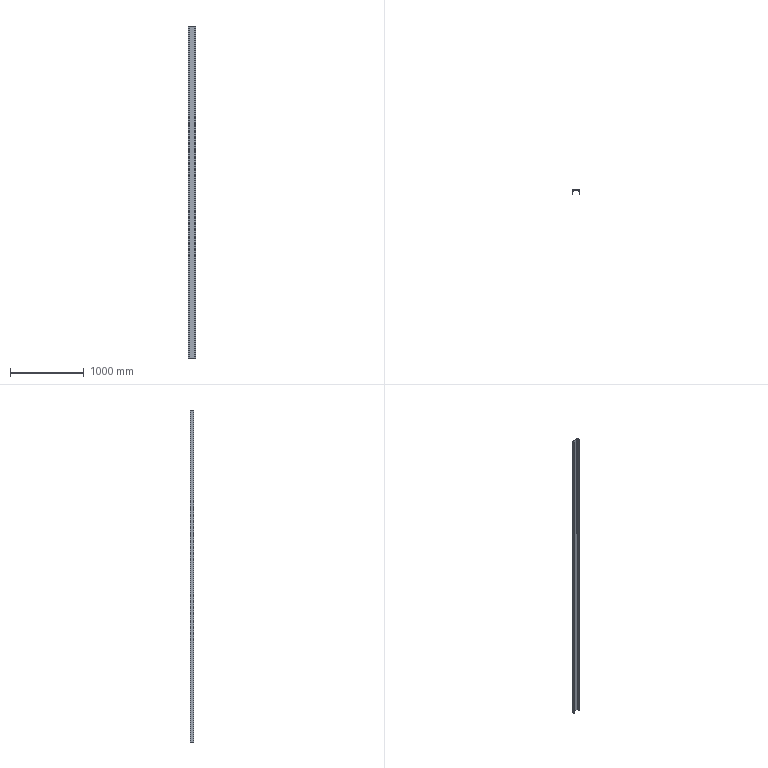Part | SolidWorks | features Extrusion 1 | 1 solid | 14 faces | box 100 x 50 x 4500 mm | volume 5749980 mm3 | plane 10 | cylinder 4 | commonest cylinder face diameters 4 x2 10 x2
STEP:
#1=CARTESIAN_POINT('',(0.,0.,0.));
#2=VERTEX_POINT('',#1);
#3=CARTESIAN_POINT('',(2.549,0.,0.));
#4=VERTEX_POINT('',#3);
#5=CARTESIAN_POINT('',(0.,0.,0.));
#6=DIRECTION('',(1.,0.,0.));
#7=VECTOR('',#6,1000.);
#8=LINE('',#5,#7);
#9=EDGE_CURVE('',#2,#4,#8,.T.);
#10=ORIENTED_EDGE('',*,*,#9,.T.);
#11=CARTESIAN_POINT('',(2.549,0.,4500.));
#12=VERTEX_POINT('',#11);
#13=CARTESIAN_POINT('',(2.549,0.,4500.));
#14=DIRECTION('',(0.,0.,-1.));
#15=VECTOR('',#14,1000.);
#16=LINE('',#13,#15);
#17=EDGE_CURVE('',#12,#4,#16,.T.);
#18=ORIENTED_EDGE('',*,*,#17,.F.);
#19=CARTESIAN_POINT('',(0.,0.,4500.));
#20=VERTEX_POINT('',#19);
#21=CARTESIAN_POINT('',(0.,0.,4500.));
#22=DIRECTION('',(1.,0.,0.));
#23=VECTOR('',#22,1000.);
#24=LINE('',#21,#23);
#25=EDGE_CURVE('',#20,#12,#24,.T.);
#26=ORIENTED_EDGE('',*,*,#25,.F.);
#27=CARTESIAN_POINT('',(0.,0.,4500.));
#28=DIRECTION('',(0.,0.,-1.));
#29=VECTOR('',#28,1000.);
#30=LINE('',#27,#29);
#31=EDGE_CURVE('',#20,#2,#30,.T.);
#32=ORIENTED_EDGE('',*,*,#31,.T.);
#33=EDGE_LOOP('',(#10,#18,#26,#32));
#34=FACE_OUTER_BOUND('',#33,.T.);
#35=CARTESIAN_POINT('',(0.,0.,4500.));
#36=DIRECTION('',(0.,1.,0.));
#37=DIRECTION('',(0.,0.,1.));
#38=AXIS2_PLACEMENT_3D('',#35,#36,#37);
#39=PLANE('',#38);
#40=ADVANCED_FACE('',(#34),#39,.F.);
#41=CARTESIAN_POINT('',(4.536,1.773,0.));
#42=VERTEX_POINT('',#41);
#43=CARTESIAN_POINT('',(2.549,2.,0.));
#44=DIRECTION('',(0.,0.,1.));
#45=DIRECTION('',(-1.,0.,0.));
#46=AXIS2_PLACEMENT_3D('',#43,#44,#45);
#47=CIRCLE('',#46,2.);
#48=EDGE_CURVE('',#4,#42,#47,.T.);
#49=ORIENTED_EDGE('',*,*,#48,.T.);
#50=CARTESIAN_POINT('',(4.536,1.773,4500.));
#51=VERTEX_POINT('',#50);
#52=CARTESIAN_POINT('',(4.536,1.773,4500.));
#53=DIRECTION('',(0.,0.,-1.));
#54=VECTOR('',#53,1000.);
#55=LINE('',#52,#54);
#56=EDGE_CURVE('',#51,#42,#55,.T.);
#57=ORIENTED_EDGE('',*,*,#56,.F.);
#58=CARTESIAN_POINT('',(2.549,2.,4500.));
#59=DIRECTION('',(0.,0.,1.));
#60=DIRECTION('',(-1.,0.,0.));
#61=AXIS2_PLACEMENT_3D('',#58,#59,#60);
#62=CIRCLE('',#61,2.);
#63=EDGE_CURVE('',#12,#51,#62,.T.);
#64=ORIENTED_EDGE('',*,*,#63,.F.);
#65=ORIENTED_EDGE('',*,*,#17,.T.);
#66=EDGE_LOOP('',(#49,#57,#64,#65));
#67=FACE_OUTER_BOUND('',#66,.T.);
#68=CARTESIAN_POINT('',(2.549,2.,4500.));
#69=DIRECTION('',(0.,0.,-1.));
#70=DIRECTION('',(-1.,0.,0.));
#71=AXIS2_PLACEMENT_3D('',#68,#69,#70);
#72=CYLINDRICAL_SURFACE('',#71,2.);
#73=ADVANCED_FACE('',(#67),#72,.T.);
#74=CARTESIAN_POINT('',(8.753,38.724,0.));
#75=VERTEX_POINT('',#74);
#76=CARTESIAN_POINT('',(4.536,1.773,0.));
#77=DIRECTION('',(0.1134,0.9936,0.));
#78=VECTOR('',#77,1000.);
#79=LINE('',#76,#78);
#80=EDGE_CURVE('',#42,#75,#79,.T.);
#81=ORIENTED_EDGE('',*,*,#80,.T.);
#82=CARTESIAN_POINT('',(8.753,38.724,4500.));
#83=VERTEX_POINT('',#82);
#84=CARTESIAN_POINT('',(8.753,38.724,4500.));
#85=DIRECTION('',(0.,0.,-1.));
#86=VECTOR('',#85,1000.);
#87=LINE('',#84,#86);
#88=EDGE_CURVE('',#83,#75,#87,.T.);
#89=ORIENTED_EDGE('',*,*,#88,.F.);
#90=CARTESIAN_POINT('',(4.536,1.773,4500.));
#91=DIRECTION('',(0.1134,0.9936,0.));
#92=VECTOR('',#91,1000.);
#93=LINE('',#90,#92);
#94=EDGE_CURVE('',#51,#83,#93,.T.);
#95=ORIENTED_EDGE('',*,*,#94,.F.);
#96=ORIENTED_EDGE('',*,*,#56,.T.);
#97=EDGE_LOOP('',(#81,#89,#95,#96));
#98=FACE_OUTER_BOUND('',#97,.T.);
#99=CARTESIAN_POINT('',(4.536,1.773,4500.));
#100=DIRECTION('',(-0.9936,0.1134,0.));
#101=DIRECTION('',(-0.1134,-0.9936,0.));
#102=AXIS2_PLACEMENT_3D('',#99,#100,#101);
#103=PLANE('',#102);
#104=ADVANCED_FACE('',(#98),#103,.F.);
#105=CARTESIAN_POINT('',(13.72,43.157,0.));
#106=VERTEX_POINT('',#105);
#107=CARTESIAN_POINT('',(13.72,38.157,0.));
#108=DIRECTION('',(0.,0.,-1.));
#109=DIRECTION('',(-1.,0.,0.));
#110=AXIS2_PLACEMENT_3D('',#107,#108,#109);
#111=CIRCLE('',#110,5.);
#112=EDGE_CURVE('',#75,#106,#111,.T.);
#113=ORIENTED_EDGE('',*,*,#112,.T.);
#114=CARTESIAN_POINT('',(13.72,43.157,4500.));
#115=VERTEX_POINT('',#114);
#116=CARTESIAN_POINT('',(13.72,43.157,4500.));
#117=DIRECTION('',(0.,0.,-1.));
#118=VECTOR('',#117,1000.);
#119=LINE('',#116,#118);
#120=EDGE_CURVE('',#115,#106,#119,.T.);
#121=ORIENTED_EDGE('',*,*,#120,.F.);
#122=CARTESIAN_POINT('',(13.72,38.157,4500.));
#123=DIRECTION('',(0.,0.,-1.));
#124=DIRECTION('',(-1.,0.,0.));
#125=AXIS2_PLACEMENT_3D('',#122,#123,#124);
#126=CIRCLE('',#125,5.);
#127=EDGE_CURVE('',#83,#115,#126,.T.);
#128=ORIENTED_EDGE('',*,*,#127,.F.);
#129=ORIENTED_EDGE('',*,*,#88,.T.);
#130=EDGE_LOOP('',(#113,#121,#128,#129));
#131=FACE_OUTER_BOUND('',#130,.T.);
#132=CARTESIAN_POINT('',(13.72,38.157,4500.));
#133=DIRECTION('',(0.,0.,-1.));
#134=DIRECTION('',(-1.,0.,0.));
#135=AXIS2_PLACEMENT_3D('',#132,#133,#134);
#136=CYLINDRICAL_SURFACE('',#135,5.);
#137=ADVANCED_FACE('',(#131),#136,.F.);
#138=CARTESIAN_POINT('',(86.28,43.157,0.));
#139=VERTEX_POINT('',#138);
#140=CARTESIAN_POINT('',(13.72,43.157,0.));
#141=DIRECTION('',(1.,0.,0.));
#142=VECTOR('',#141,1000.);
#143=LINE('',#140,#142);
#144=EDGE_CURVE('',#106,#139,#143,.T.);
#145=ORIENTED_EDGE('',*,*,#144,.T.);
#146=CARTESIAN_POINT('',(86.28,43.157,4500.));
#147=VERTEX_POINT('',#146);
#148=CARTESIAN_POINT('',(86.28,43.157,4500.));
#149=DIRECTION('',(0.,0.,-1.));
#150=VECTOR('',#149,1000.);
#151=LINE('',#148,#150);
#152=EDGE_CURVE('',#147,#139,#151,.T.);
#153=ORIENTED_EDGE('',*,*,#152,.F.);
#154=CARTESIAN_POINT('',(13.72,43.157,4500.));
#155=DIRECTION('',(1.,0.,0.));
#156=VECTOR('',#155,1000.);
#157=LINE('',#154,#156);
#158=EDGE_CURVE('',#115,#147,#157,.T.);
#159=ORIENTED_EDGE('',*,*,#158,.F.);
#160=ORIENTED_EDGE('',*,*,#120,.T.);
#161=EDGE_LOOP('',(#145,#153,#159,#160));
#162=FACE_OUTER_BOUND('',#161,.T.);
#163=CARTESIAN_POINT('',(13.72,43.157,4500.));
#164=DIRECTION('',(0.,1.,0.));
#165=DIRECTION('',(-1.,0.,0.));
#166=AXIS2_PLACEMENT_3D('',#163,#164,#165);
#167=PLANE('',#166);
#168=ADVANCED_FACE('',(#162),#167,.F.);
#169=CARTESIAN_POINT('',(91.247,38.724,0.));
#170=VERTEX_POINT('',#169);
#171=CARTESIAN_POINT('',(86.28,38.157,0.));
#172=DIRECTION('',(0.,0.,-1.));
#173=DIRECTION('',(1.,0.,0.));
#174=AXIS2_PLACEMENT_3D('',#171,#172,#173);
#175=CIRCLE('',#174,5.);
#176=EDGE_CURVE('',#139,#170,#175,.T.);
#177=ORIENTED_EDGE('',*,*,#176,.T.);
#178=CARTESIAN_POINT('',(91.247,38.724,4500.));
#179=VERTEX_POINT('',#178);
#180=CARTESIAN_POINT('',(91.247,38.724,4500.));
#181=DIRECTION('',(0.,0.,-1.));
#182=VECTOR('',#181,1000.);
#183=LINE('',#180,#182);
#184=EDGE_CURVE('',#179,#170,#183,.T.);
#185=ORIENTED_EDGE('',*,*,#184,.F.);
#186=CARTESIAN_POINT('',(86.28,38.157,4500.));
#187=DIRECTION('',(0.,0.,-1.));
#188=DIRECTION('',(1.,0.,0.));
#189=AXIS2_PLACEMENT_3D('',#186,#187,#188);
#190=CIRCLE('',#189,5.);
#191=EDGE_CURVE('',#147,#179,#190,.T.);
#192=ORIENTED_EDGE('',*,*,#191,.F.);
#193=ORIENTED_EDGE('',*,*,#152,.T.);
#194=EDGE_LOOP('',(#177,#185,#192,#193));
#195=FACE_OUTER_BOUND('',#194,.T.);
#196=CARTESIAN_POINT('',(86.28,38.157,4500.));
#197=DIRECTION('',(0.,0.,-1.));
#198=DIRECTION('',(-1.,0.,0.));
#199=AXIS2_PLACEMENT_3D('',#196,#197,#198);
#200=CYLINDRICAL_SURFACE('',#199,5.);
#201=ADVANCED_FACE('',(#195),#200,.F.);
#202=CARTESIAN_POINT('',(95.464,1.773,0.));
#203=VERTEX_POINT('',#202);
#204=CARTESIAN_POINT('',(95.464,1.773,0.));
#205=DIRECTION('',(0.1134,-0.9936,0.));
#206=VECTOR('',#205,1000.);
#207=LINE('',#204,#206);
#208=EDGE_CURVE('',#170,#203,#207,.T.);
#209=ORIENTED_EDGE('',*,*,#208,.T.);
#210=CARTESIAN_POINT('',(95.464,1.773,4500.));
#211=VERTEX_POINT('',#210);
#212=CARTESIAN_POINT('',(95.464,1.773,4500.));
#213=DIRECTION('',(0.,0.,-1.));
#214=VECTOR('',#213,1000.);
#215=LINE('',#212,#214);
#216=EDGE_CURVE('',#211,#203,#215,.T.);
#217=ORIENTED_EDGE('',*,*,#216,.F.);
#218=CARTESIAN_POINT('',(95.464,1.773,4500.));
#219=DIRECTION('',(0.1134,-0.9936,0.));
#220=VECTOR('',#219,1000.);
#221=LINE('',#218,#220);
#222=EDGE_CURVE('',#179,#211,#221,.T.);
#223=ORIENTED_EDGE('',*,*,#222,.F.);
#224=ORIENTED_EDGE('',*,*,#184,.T.);
#225=EDGE_LOOP('',(#209,#217,#223,#224));
#226=FACE_OUTER_BOUND('',#225,.T.);
#227=CARTESIAN_POINT('',(95.464,1.773,4500.));
#228=DIRECTION('',(0.9936,0.1134,0.));
#229=DIRECTION('',(-0.1134,0.9936,0.));
#230=AXIS2_PLACEMENT_3D('',#227,#228,#229);
#231=PLANE('',#230);
#232=ADVANCED_FACE('',(#226),#231,.F.);
#233=CARTESIAN_POINT('',(97.451,0.,0.));
#234=VERTEX_POINT('',#233);
#235=CARTESIAN_POINT('',(97.451,2.,0.));
#236=DIRECTION('',(0.,0.,1.));
#237=DIRECTION('',(1.,0.,0.));
#238=AXIS2_PLACEMENT_3D('',#235,#236,#237);
#239=CIRCLE('',#238,2.);
#240=EDGE_CURVE('',#203,#234,#239,.T.);
#241=ORIENTED_EDGE('',*,*,#240,.T.);
#242=CARTESIAN_POINT('',(97.451,0.,4500.));
#243=VERTEX_POINT('',#242);
#244=CARTESIAN_POINT('',(97.451,0.,4500.));
#245=DIRECTION('',(0.,0.,-1.));
#246=VECTOR('',#245,1000.);
#247=LINE('',#244,#246);
#248=EDGE_CURVE('',#243,#234,#247,.T.);
#249=ORIENTED_EDGE('',*,*,#248,.F.);
#250=CARTESIAN_POINT('',(97.451,2.,4500.));
#251=DIRECTION('',(0.,0.,1.));
#252=DIRECTION('',(1.,0.,0.));
#253=AXIS2_PLACEMENT_3D('',#250,#251,#252);
#254=CIRCLE('',#253,2.);
#255=EDGE_CURVE('',#211,#243,#254,.T.);
#256=ORIENTED_EDGE('',*,*,#255,.F.);
#257=ORIENTED_EDGE('',*,*,#216,.T.);
#258=EDGE_LOOP('',(#241,#249,#256,#257));
#259=FACE_OUTER_BOUND('',#258,.T.);
#260=CARTESIAN_POINT('',(97.451,2.,4500.));
#261=DIRECTION('',(0.,0.,-1.));
#262=DIRECTION('',(-1.,0.,0.));
#263=AXIS2_PLACEMENT_3D('',#260,#261,#262);
#264=CYLINDRICAL_SURFACE('',#263,2.);
#265=ADVANCED_FACE('',(#259),#264,.T.);
#266=CARTESIAN_POINT('',(100.,0.,0.));
#267=VERTEX_POINT('',#266);
#268=CARTESIAN_POINT('',(100.,0.,0.));
#269=DIRECTION('',(1.,0.,0.));
#270=VECTOR('',#269,1000.);
#271=LINE('',#268,#270);
#272=EDGE_CURVE('',#234,#267,#271,.T.);
#273=ORIENTED_EDGE('',*,*,#272,.T.);
#274=CARTESIAN_POINT('',(100.,0.,4500.));
#275=VERTEX_POINT('',#274);
#276=CARTESIAN_POINT('',(100.,0.,4500.));
#277=DIRECTION('',(0.,0.,-1.));
#278=VECTOR('',#277,1000.);
#279=LINE('',#276,#278);
#280=EDGE_CURVE('',#275,#267,#279,.T.);
#281=ORIENTED_EDGE('',*,*,#280,.F.);
#282=CARTESIAN_POINT('',(100.,0.,4500.));
#283=DIRECTION('',(1.,0.,0.));
#284=VECTOR('',#283,1000.);
#285=LINE('',#282,#284);
#286=EDGE_CURVE('',#243,#275,#285,.T.);
#287=ORIENTED_EDGE('',*,*,#286,.F.);
#288=ORIENTED_EDGE('',*,*,#248,.T.);
#289=EDGE_LOOP('',(#273,#281,#287,#288));
#290=FACE_OUTER_BOUND('',#289,.T.);
#291=CARTESIAN_POINT('',(100.,0.,4500.));
#292=DIRECTION('',(0.,1.,0.));
#293=DIRECTION('',(-1.,0.,0.));
#294=AXIS2_PLACEMENT_3D('',#291,#292,#293);
#295=PLANE('',#294);
#296=ADVANCED_FACE('',(#290),#295,.F.);
#297=CARTESIAN_POINT('',(100.,50.,0.));
#298=VERTEX_POINT('',#297);
#299=CARTESIAN_POINT('',(100.,50.,0.));
#300=DIRECTION('',(0.,1.,0.));
#301=VECTOR('',#300,1000.);
#302=LINE('',#299,#301);
#303=EDGE_CURVE('',#267,#298,#302,.T.);
#304=ORIENTED_EDGE('',*,*,#303,.T.);
#305=CARTESIAN_POINT('',(100.,50.,4500.));
#306=VERTEX_POINT('',#305);
#307=CARTESIAN_POINT('',(100.,50.,4500.));
#308=DIRECTION('',(0.,0.,-1.));
#309=VECTOR('',#308,1000.);
#310=LINE('',#307,#309);
#311=EDGE_CURVE('',#306,#298,#310,.T.);
#312=ORIENTED_EDGE('',*,*,#311,.F.);
#313=CARTESIAN_POINT('',(100.,50.,4500.));
#314=DIRECTION('',(0.,1.,0.));
#315=VECTOR('',#314,1000.);
#316=LINE('',#313,#315);
#317=EDGE_CURVE('',#275,#306,#316,.T.);
#318=ORIENTED_EDGE('',*,*,#317,.F.);
#319=ORIENTED_EDGE('',*,*,#280,.T.);
#320=EDGE_LOOP('',(#304,#312,#318,#319));
#321=FACE_OUTER_BOUND('',#320,.T.);
#322=CARTESIAN_POINT('',(100.,50.,4500.));
#323=DIRECTION('',(-1.,0.,0.));
#324=DIRECTION('',(0.,-1.,0.));
#325=AXIS2_PLACEMENT_3D('',#322,#323,#324);
#326=PLANE('',#325);
#327=ADVANCED_FACE('',(#321),#326,.F.);
#328=CARTESIAN_POINT('',(0.,50.,0.));
#329=VERTEX_POINT('',#328);
#330=CARTESIAN_POINT('',(0.,50.,0.));
#331=DIRECTION('',(-1.,0.,0.));
#332=VECTOR('',#331,1000.);
#333=LINE('',#330,#332);
#334=EDGE_CURVE('',#298,#329,#333,.T.);
#335=ORIENTED_EDGE('',*,*,#334,.T.);
#336=CARTESIAN_POINT('',(0.,50.,4500.));
#337=VERTEX_POINT('',#336);
#338=CARTESIAN_POINT('',(0.,50.,4500.));
#339=DIRECTION('',(0.,0.,-1.));
#340=VECTOR('',#339,1000.);
#341=LINE('',#338,#340);
#342=EDGE_CURVE('',#337,#329,#341,.T.);
#343=ORIENTED_EDGE('',*,*,#342,.F.);
#344=CARTESIAN_POINT('',(0.,50.,4500.));
#345=DIRECTION('',(-1.,0.,0.));
#346=VECTOR('',#345,1000.);
#347=LINE('',#344,#346);
#348=EDGE_CURVE('',#306,#337,#347,.T.);
#349=ORIENTED_EDGE('',*,*,#348,.F.);
#350=ORIENTED_EDGE('',*,*,#311,.T.);
#351=EDGE_LOOP('',(#335,#343,#349,#350));
#352=FACE_OUTER_BOUND('',#351,.T.);
#353=CARTESIAN_POINT('',(0.,50.,4500.));
#354=DIRECTION('',(0.,-1.,0.));
#355=DIRECTION('',(1.,0.,0.));
#356=AXIS2_PLACEMENT_3D('',#353,#354,#355);
#357=PLANE('',#356);
#358=ADVANCED_FACE('',(#352),#357,.F.);
#359=CARTESIAN_POINT('',(0.,0.,0.));
#360=DIRECTION('',(0.,-1.,0.));
#361=VECTOR('',#360,1000.);
#362=LINE('',#359,#361);
#363=EDGE_CURVE('',#329,#2,#362,.T.);
#364=ORIENTED_EDGE('',*,*,#363,.T.);
#365=ORIENTED_EDGE('',*,*,#31,.F.);
#366=CARTESIAN_POINT('',(0.,0.,4500.));
#367=DIRECTION('',(0.,-1.,0.));
#368=VECTOR('',#367,1000.);
#369=LINE('',#366,#368);
#370=EDGE_CURVE('',#337,#20,#369,.T.);
#371=ORIENTED_EDGE('',*,*,#370,.F.);
#372=ORIENTED_EDGE('',*,*,#342,.T.);
#373=EDGE_LOOP('',(#364,#365,#371,#372));
#374=FACE_OUTER_BOUND('',#373,.T.);
#375=CARTESIAN_POINT('',(0.,0.,4500.));
#376=DIRECTION('',(1.,0.,0.));
#377=DIRECTION('',(0.,0.,-1.));
#378=AXIS2_PLACEMENT_3D('',#375,#376,#377);
#379=PLANE('',#378);
#380=ADVANCED_FACE('',(#374),#379,.F.);
#381=ORIENTED_EDGE('',*,*,#25,.T.);
#382=ORIENTED_EDGE('',*,*,#63,.T.);
#383=ORIENTED_EDGE('',*,*,#94,.T.);
#384=ORIENTED_EDGE('',*,*,#127,.T.);
#385=ORIENTED_EDGE('',*,*,#158,.T.);
#386=ORIENTED_EDGE('',*,*,#191,.T.);
#387=ORIENTED_EDGE('',*,*,#222,.T.);
#388=ORIENTED_EDGE('',*,*,#255,.T.);
#389=ORIENTED_EDGE('',*,*,#286,.T.);
#390=ORIENTED_EDGE('',*,*,#317,.T.);
#391=ORIENTED_EDGE('',*,*,#348,.T.);
#392=ORIENTED_EDGE('',*,*,#370,.T.);
#393=EDGE_LOOP('',(#381,#382,#383,#384,#385,#386,#387,#388,#389,#390,#391,#392));
#394=FACE_OUTER_BOUND('',#393,.T.);
#395=CARTESIAN_POINT('',(2.549,2.,4500.));
#396=DIRECTION('',(0.,0.,-1.));
#397=DIRECTION('',(-1.,0.,0.));
#398=AXIS2_PLACEMENT_3D('',#395,#396,#397);
#399=PLANE('',#398);
#400=ADVANCED_FACE('',(#394),#399,.F.);
#401=ORIENTED_EDGE('',*,*,#9,.F.);
#402=ORIENTED_EDGE('',*,*,#363,.F.);
#403=ORIENTED_EDGE('',*,*,#334,.F.);
#404=ORIENTED_EDGE('',*,*,#303,.F.);
#405=ORIENTED_EDGE('',*,*,#272,.F.);
#406=ORIENTED_EDGE('',*,*,#240,.F.);
#407=ORIENTED_EDGE('',*,*,#208,.F.);
#408=ORIENTED_EDGE('',*,*,#176,.F.);
#409=ORIENTED_EDGE('',*,*,#144,.F.);
#410=ORIENTED_EDGE('',*,*,#112,.F.);
#411=ORIENTED_EDGE('',*,*,#80,.F.);
#412=ORIENTED_EDGE('',*,*,#48,.F.);
#413=EDGE_LOOP('',(#401,#402,#403,#404,#405,#406,#407,#408,#409,#410,#411,#412));
#414=FACE_OUTER_BOUND('',#413,.T.);
#415=CARTESIAN_POINT('',(2.549,2.,0.));
#416=DIRECTION('',(0.,0.,-1.));
#417=DIRECTION('',(-1.,0.,0.));
#418=AXIS2_PLACEMENT_3D('',#415,#416,#417);
#419=PLANE('',#418);
#420=ADVANCED_FACE('',(#414),#419,.T.);
#421=CLOSED_SHELL('',(#40,#73,#104,#137,#168,#201,#232,#265,#296,#327,#358,#380,#400,#420));
#422=MANIFOLD_SOLID_BREP('',#421);
#423=CARTESIAN_POINT('',(0.,0.,0.));
#424=DIRECTION('',(0.,0.,1.));
#425=DIRECTION('',(1.,0.,0.));
#426=AXIS2_PLACEMENT_3D('',#423,#424,#425);
#427=(LENGTH_UNIT()NAMED_UNIT(*)SI_UNIT(.MILLI.,.METRE.));
#428=UNCERTAINTY_MEASURE_WITH_UNIT(LENGTH_MEASURE(0.00001),#427,'','');
#429=(NAMED_UNIT(*)PLANE_ANGLE_UNIT()SI_UNIT($,.RADIAN.));
#430=(NAMED_UNIT(*)SI_UNIT($,.STERADIAN.)SOLID_ANGLE_UNIT());
#431=(GEOMETRIC_REPRESENTATION_CONTEXT(3)GLOBAL_UNCERTAINTY_ASSIGNED_CONTEXT((#428))GLOBAL_UNIT_ASSIGNED_CONTEXT((#427,#429,#430))REPRESENTATION_CONTEXT('',''));
#432=ADVANCED_BREP_SHAPE_REPRESENTATION('',(#422,#426),#431);